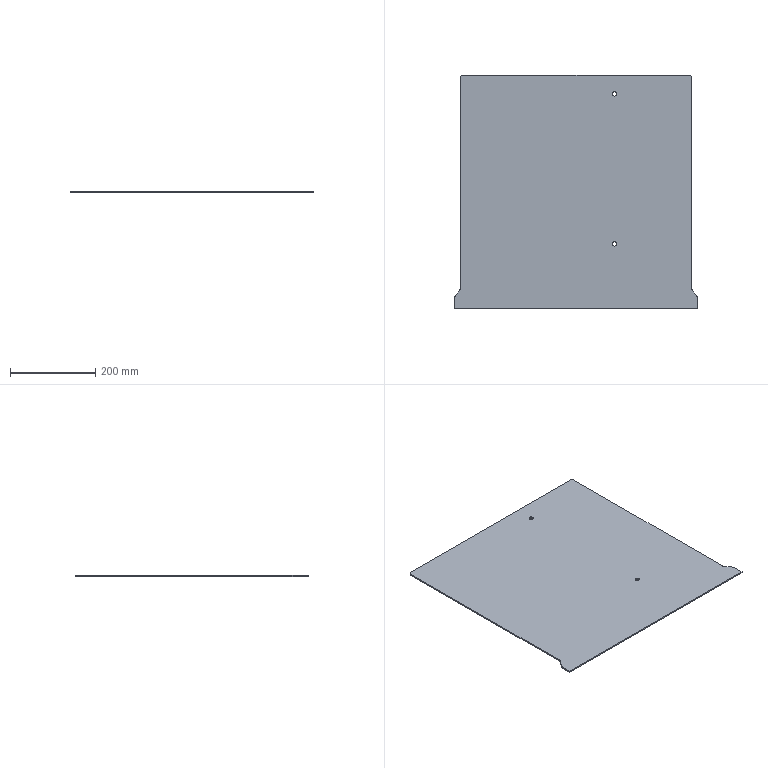Part | SolidWorks | features Fillet 2, FlatPattern 1, SMBaseFlange 1, SheetMetal 1 | 1 solid | 20 faces | box 570 x 547 x 3 mm | volume 888967 mm3 | cylinder 10 | plane 10 | commonest cylinder face diameters 10 x6 20 x4
STEP:
#1=CARTESIAN_POINT('',(370.,152.,-3.));
#2=VERTEX_POINT('',#1);
#3=CARTESIAN_POINT('',(380.,152.,-3.));
#4=VERTEX_POINT('',#3);
#5=CARTESIAN_POINT('',(375.,152.,-3.));
#6=DIRECTION('',(0.,0.,1.));
#7=DIRECTION('',(1.,0.,0.));
#8=AXIS2_PLACEMENT_3D('',#5,#6,#7);
#9=CIRCLE('',#8,5.);
#10=EDGE_CURVE('',#2,#4,#9,.T.);
#11=ORIENTED_EDGE('',*,*,#10,.F.);
#12=CARTESIAN_POINT('',(370.,152.,0.));
#13=VERTEX_POINT('',#12);
#14=CARTESIAN_POINT('',(370.,152.,-3.));
#15=DIRECTION('',(0.,0.,1.));
#16=VECTOR('',#15,1000.);
#17=LINE('',#14,#16);
#18=EDGE_CURVE('',#2,#13,#17,.T.);
#19=ORIENTED_EDGE('',*,*,#18,.T.);
#20=CARTESIAN_POINT('',(380.,152.,0.));
#21=VERTEX_POINT('',#20);
#22=CARTESIAN_POINT('',(375.,152.,0.));
#23=DIRECTION('',(0.,0.,1.));
#24=DIRECTION('',(1.,0.,0.));
#25=AXIS2_PLACEMENT_3D('',#22,#23,#24);
#26=CIRCLE('',#25,5.);
#27=EDGE_CURVE('',#13,#21,#26,.T.);
#28=ORIENTED_EDGE('',*,*,#27,.T.);
#29=CARTESIAN_POINT('',(380.,152.,-3.));
#30=DIRECTION('',(0.,0.,1.));
#31=VECTOR('',#30,1000.);
#32=LINE('',#29,#31);
#33=EDGE_CURVE('',#4,#21,#32,.T.);
#34=ORIENTED_EDGE('',*,*,#33,.F.);
#35=EDGE_LOOP('',(#11,#19,#28,#34));
#36=FACE_OUTER_BOUND('',#35,.T.);
#37=CARTESIAN_POINT('',(375.,152.,-3.));
#38=DIRECTION('',(0.,0.,1.));
#39=DIRECTION('',(1.,0.,0.));
#40=AXIS2_PLACEMENT_3D('',#37,#38,#39);
#41=CYLINDRICAL_SURFACE('',#40,5.);
#42=ADVANCED_FACE('',(#36),#41,.F.);
#43=CARTESIAN_POINT('',(370.,503.,-3.));
#44=VERTEX_POINT('',#43);
#45=CARTESIAN_POINT('',(380.,503.,-3.));
#46=VERTEX_POINT('',#45);
#47=CARTESIAN_POINT('',(375.,503.,-3.));
#48=DIRECTION('',(0.,0.,1.));
#49=DIRECTION('',(1.,0.,0.));
#50=AXIS2_PLACEMENT_3D('',#47,#48,#49);
#51=CIRCLE('',#50,5.);
#52=EDGE_CURVE('',#44,#46,#51,.T.);
#53=ORIENTED_EDGE('',*,*,#52,.F.);
#54=CARTESIAN_POINT('',(370.,503.,0.));
#55=VERTEX_POINT('',#54);
#56=CARTESIAN_POINT('',(370.,503.,-3.));
#57=DIRECTION('',(0.,0.,1.));
#58=VECTOR('',#57,1000.);
#59=LINE('',#56,#58);
#60=EDGE_CURVE('',#44,#55,#59,.T.);
#61=ORIENTED_EDGE('',*,*,#60,.T.);
#62=CARTESIAN_POINT('',(380.,503.,0.));
#63=VERTEX_POINT('',#62);
#64=CARTESIAN_POINT('',(375.,503.,0.));
#65=DIRECTION('',(0.,0.,1.));
#66=DIRECTION('',(1.,0.,0.));
#67=AXIS2_PLACEMENT_3D('',#64,#65,#66);
#68=CIRCLE('',#67,5.);
#69=EDGE_CURVE('',#55,#63,#68,.T.);
#70=ORIENTED_EDGE('',*,*,#69,.T.);
#71=CARTESIAN_POINT('',(380.,503.,-3.));
#72=DIRECTION('',(0.,0.,1.));
#73=VECTOR('',#72,1000.);
#74=LINE('',#71,#73);
#75=EDGE_CURVE('',#46,#63,#74,.T.);
#76=ORIENTED_EDGE('',*,*,#75,.F.);
#77=EDGE_LOOP('',(#53,#61,#70,#76));
#78=FACE_OUTER_BOUND('',#77,.T.);
#79=CARTESIAN_POINT('',(375.,503.,-3.));
#80=DIRECTION('',(0.,0.,1.));
#81=DIRECTION('',(1.,0.,0.));
#82=AXIS2_PLACEMENT_3D('',#79,#80,#81);
#83=CYLINDRICAL_SURFACE('',#82,5.);
#84=ADVANCED_FACE('',(#78),#83,.F.);
#85=CARTESIAN_POINT('',(0.,23.667,0.));
#86=VERTEX_POINT('',#85);
#87=CARTESIAN_POINT('',(0.,0.,0.));
#88=VERTEX_POINT('',#87);
#89=CARTESIAN_POINT('',(0.,0.,0.));
#90=DIRECTION('',(0.,-1.,0.));
#91=VECTOR('',#90,1000.);
#92=LINE('',#89,#91);
#93=EDGE_CURVE('',#86,#88,#92,.T.);
#94=ORIENTED_EDGE('',*,*,#93,.F.);
#95=CARTESIAN_POINT('',(0.,23.667,-3.));
#96=VERTEX_POINT('',#95);
#97=CARTESIAN_POINT('',(0.,23.667,-3.));
#98=DIRECTION('',(0.,0.,-1.));
#99=VECTOR('',#98,1000.);
#100=LINE('',#97,#99);
#101=EDGE_CURVE('',#86,#96,#100,.T.);
#102=ORIENTED_EDGE('',*,*,#101,.T.);
#103=CARTESIAN_POINT('',(0.,0.,-3.));
#104=VERTEX_POINT('',#103);
#105=CARTESIAN_POINT('',(0.,0.,-3.));
#106=DIRECTION('',(0.,-1.,0.));
#107=VECTOR('',#106,1000.);
#108=LINE('',#105,#107);
#109=EDGE_CURVE('',#96,#104,#108,.T.);
#110=ORIENTED_EDGE('',*,*,#109,.T.);
#111=CARTESIAN_POINT('',(0.,0.,-3.));
#112=DIRECTION('',(0.,0.,1.));
#113=VECTOR('',#112,1000.);
#114=LINE('',#111,#113);
#115=EDGE_CURVE('',#104,#88,#114,.T.);
#116=ORIENTED_EDGE('',*,*,#115,.T.);
#117=EDGE_LOOP('',(#94,#102,#110,#116));
#118=FACE_OUTER_BOUND('',#117,.T.);
#119=CARTESIAN_POINT('',(0.,0.,-3.));
#120=DIRECTION('',(-1.,0.,0.));
#121=DIRECTION('',(0.,0.,1.));
#122=AXIS2_PLACEMENT_3D('',#119,#120,#121);
#123=PLANE('',#122);
#124=ADVANCED_FACE('',(#118),#123,.T.);
#125=CARTESIAN_POINT('',(13.,44.333,-3.));
#126=VERTEX_POINT('',#125);
#127=CARTESIAN_POINT('',(2.,29.667,-3.));
#128=VERTEX_POINT('',#127);
#129=CARTESIAN_POINT('',(15.,47.,-3.));
#130=DIRECTION('',(-0.6,-0.8,0.));
#131=VECTOR('',#130,1000.);
#132=LINE('',#129,#131);
#133=EDGE_CURVE('',#126,#128,#132,.T.);
#134=ORIENTED_EDGE('',*,*,#133,.T.);
#135=CARTESIAN_POINT('',(2.,29.667,0.));
#136=VERTEX_POINT('',#135);
#137=CARTESIAN_POINT('',(2.,29.667,-3.));
#138=DIRECTION('',(0.,0.,1.));
#139=VECTOR('',#138,1000.);
#140=LINE('',#137,#139);
#141=EDGE_CURVE('',#128,#136,#140,.T.);
#142=ORIENTED_EDGE('',*,*,#141,.T.);
#143=CARTESIAN_POINT('',(13.,44.333,0.));
#144=VERTEX_POINT('',#143);
#145=CARTESIAN_POINT('',(15.,47.,0.));
#146=DIRECTION('',(-0.6,-0.8,0.));
#147=VECTOR('',#146,1000.);
#148=LINE('',#145,#147);
#149=EDGE_CURVE('',#144,#136,#148,.T.);
#150=ORIENTED_EDGE('',*,*,#149,.F.);
#151=CARTESIAN_POINT('',(13.,44.333,-3.));
#152=DIRECTION('',(0.,0.,-1.));
#153=VECTOR('',#152,1000.);
#154=LINE('',#151,#153);
#155=EDGE_CURVE('',#144,#126,#154,.T.);
#156=ORIENTED_EDGE('',*,*,#155,.T.);
#157=EDGE_LOOP('',(#134,#142,#150,#156));
#158=FACE_OUTER_BOUND('',#157,.T.);
#159=CARTESIAN_POINT('',(15.,47.,-3.));
#160=DIRECTION('',(-0.8,0.6,0.));
#161=DIRECTION('',(-0.6,-0.8,0.));
#162=AXIS2_PLACEMENT_3D('',#159,#160,#161);
#163=PLANE('',#162);
#164=ADVANCED_FACE('',(#158),#163,.T.);
#165=CARTESIAN_POINT('',(15.,542.,0.));
#166=VERTEX_POINT('',#165);
#167=CARTESIAN_POINT('',(15.,50.333,0.));
#168=VERTEX_POINT('',#167);
#169=CARTESIAN_POINT('',(15.,547.,0.));
#170=DIRECTION('',(0.,-1.,0.));
#171=VECTOR('',#170,1000.);
#172=LINE('',#169,#171);
#173=EDGE_CURVE('',#166,#168,#172,.T.);
#174=ORIENTED_EDGE('',*,*,#173,.F.);
#175=CARTESIAN_POINT('',(15.,542.,-3.));
#176=VERTEX_POINT('',#175);
#177=CARTESIAN_POINT('',(15.,542.,-3.));
#178=DIRECTION('',(0.,0.,-1.));
#179=VECTOR('',#178,1000.);
#180=LINE('',#177,#179);
#181=EDGE_CURVE('',#166,#176,#180,.T.);
#182=ORIENTED_EDGE('',*,*,#181,.T.);
#183=CARTESIAN_POINT('',(15.,50.333,-3.));
#184=VERTEX_POINT('',#183);
#185=CARTESIAN_POINT('',(15.,547.,-3.));
#186=DIRECTION('',(0.,-1.,0.));
#187=VECTOR('',#186,1000.);
#188=LINE('',#185,#187);
#189=EDGE_CURVE('',#176,#184,#188,.T.);
#190=ORIENTED_EDGE('',*,*,#189,.T.);
#191=CARTESIAN_POINT('',(15.,50.333,0.));
#192=DIRECTION('',(0.,0.,1.));
#193=VECTOR('',#192,1000.);
#194=LINE('',#191,#193);
#195=EDGE_CURVE('',#184,#168,#194,.T.);
#196=ORIENTED_EDGE('',*,*,#195,.T.);
#197=EDGE_LOOP('',(#174,#182,#190,#196));
#198=FACE_OUTER_BOUND('',#197,.T.);
#199=CARTESIAN_POINT('',(15.,547.,-3.));
#200=DIRECTION('',(-1.,0.,0.));
#201=DIRECTION('',(0.,-1.,0.));
#202=AXIS2_PLACEMENT_3D('',#199,#200,#201);
#203=PLANE('',#202);
#204=ADVANCED_FACE('',(#198),#203,.T.);
#205=CARTESIAN_POINT('',(550.,547.,0.));
#206=VERTEX_POINT('',#205);
#207=CARTESIAN_POINT('',(20.,547.,0.));
#208=VERTEX_POINT('',#207);
#209=CARTESIAN_POINT('',(15.,547.,0.));
#210=DIRECTION('',(-1.,0.,0.));
#211=VECTOR('',#210,1000.);
#212=LINE('',#209,#211);
#213=EDGE_CURVE('',#206,#208,#212,.T.);
#214=ORIENTED_EDGE('',*,*,#213,.F.);
#215=CARTESIAN_POINT('',(550.,547.,-3.));
#216=VERTEX_POINT('',#215);
#217=CARTESIAN_POINT('',(550.,547.,-3.));
#218=DIRECTION('',(0.,0.,-1.));
#219=VECTOR('',#218,1000.);
#220=LINE('',#217,#219);
#221=EDGE_CURVE('',#206,#216,#220,.T.);
#222=ORIENTED_EDGE('',*,*,#221,.T.);
#223=CARTESIAN_POINT('',(20.,547.,-3.));
#224=VERTEX_POINT('',#223);
#225=CARTESIAN_POINT('',(15.,547.,-3.));
#226=DIRECTION('',(-1.,0.,0.));
#227=VECTOR('',#226,1000.);
#228=LINE('',#225,#227);
#229=EDGE_CURVE('',#216,#224,#228,.T.);
#230=ORIENTED_EDGE('',*,*,#229,.T.);
#231=CARTESIAN_POINT('',(20.,547.,-3.));
#232=DIRECTION('',(0.,0.,1.));
#233=VECTOR('',#232,1000.);
#234=LINE('',#231,#233);
#235=EDGE_CURVE('',#224,#208,#234,.T.);
#236=ORIENTED_EDGE('',*,*,#235,.T.);
#237=EDGE_LOOP('',(#214,#222,#230,#236));
#238=FACE_OUTER_BOUND('',#237,.T.);
#239=CARTESIAN_POINT('',(15.,547.,-3.));
#240=DIRECTION('',(0.,1.,0.));
#241=DIRECTION('',(-1.,0.,0.));
#242=AXIS2_PLACEMENT_3D('',#239,#240,#241);
#243=PLANE('',#242);
#244=ADVANCED_FACE('',(#238),#243,.T.);
#245=CARTESIAN_POINT('',(555.,50.333,-3.));
#246=VERTEX_POINT('',#245);
#247=CARTESIAN_POINT('',(555.,542.,-3.));
#248=VERTEX_POINT('',#247);
#249=CARTESIAN_POINT('',(555.,547.,-3.));
#250=DIRECTION('',(0.,1.,0.));
#251=VECTOR('',#250,1000.);
#252=LINE('',#249,#251);
#253=EDGE_CURVE('',#246,#248,#252,.T.);
#254=ORIENTED_EDGE('',*,*,#253,.T.);
#255=CARTESIAN_POINT('',(555.,542.,0.));
#256=VERTEX_POINT('',#255);
#257=CARTESIAN_POINT('',(555.,542.,-3.));
#258=DIRECTION('',(0.,0.,1.));
#259=VECTOR('',#258,1000.);
#260=LINE('',#257,#259);
#261=EDGE_CURVE('',#248,#256,#260,.T.);
#262=ORIENTED_EDGE('',*,*,#261,.T.);
#263=CARTESIAN_POINT('',(555.,50.333,0.));
#264=VERTEX_POINT('',#263);
#265=CARTESIAN_POINT('',(555.,547.,0.));
#266=DIRECTION('',(0.,1.,0.));
#267=VECTOR('',#266,1000.);
#268=LINE('',#265,#267);
#269=EDGE_CURVE('',#264,#256,#268,.T.);
#270=ORIENTED_EDGE('',*,*,#269,.F.);
#271=CARTESIAN_POINT('',(555.,50.333,-3.));
#272=DIRECTION('',(0.,0.,-1.));
#273=VECTOR('',#272,1000.);
#274=LINE('',#271,#273);
#275=EDGE_CURVE('',#264,#246,#274,.T.);
#276=ORIENTED_EDGE('',*,*,#275,.T.);
#277=EDGE_LOOP('',(#254,#262,#270,#276));
#278=FACE_OUTER_BOUND('',#277,.T.);
#279=CARTESIAN_POINT('',(555.,547.,-3.));
#280=DIRECTION('',(1.,0.,0.));
#281=DIRECTION('',(0.,1.,0.));
#282=AXIS2_PLACEMENT_3D('',#279,#280,#281);
#283=PLANE('',#282);
#284=ADVANCED_FACE('',(#278),#283,.T.);
#285=CARTESIAN_POINT('',(568.,29.667,0.));
#286=VERTEX_POINT('',#285);
#287=CARTESIAN_POINT('',(557.,44.333,0.));
#288=VERTEX_POINT('',#287);
#289=CARTESIAN_POINT('',(555.,47.,0.));
#290=DIRECTION('',(-0.6,0.8,0.));
#291=VECTOR('',#290,1000.);
#292=LINE('',#289,#291);
#293=EDGE_CURVE('',#286,#288,#292,.T.);
#294=ORIENTED_EDGE('',*,*,#293,.F.);
#295=CARTESIAN_POINT('',(568.,29.667,-3.));
#296=VERTEX_POINT('',#295);
#297=CARTESIAN_POINT('',(568.,29.667,-3.));
#298=DIRECTION('',(0.,0.,-1.));
#299=VECTOR('',#298,1000.);
#300=LINE('',#297,#299);
#301=EDGE_CURVE('',#286,#296,#300,.T.);
#302=ORIENTED_EDGE('',*,*,#301,.T.);
#303=CARTESIAN_POINT('',(557.,44.333,-3.));
#304=VERTEX_POINT('',#303);
#305=CARTESIAN_POINT('',(555.,47.,-3.));
#306=DIRECTION('',(-0.6,0.8,0.));
#307=VECTOR('',#306,1000.);
#308=LINE('',#305,#307);
#309=EDGE_CURVE('',#296,#304,#308,.T.);
#310=ORIENTED_EDGE('',*,*,#309,.T.);
#311=CARTESIAN_POINT('',(557.,44.333,0.));
#312=DIRECTION('',(0.,0.,1.));
#313=VECTOR('',#312,1000.);
#314=LINE('',#311,#313);
#315=EDGE_CURVE('',#304,#288,#314,.T.);
#316=ORIENTED_EDGE('',*,*,#315,.T.);
#317=EDGE_LOOP('',(#294,#302,#310,#316));
#318=FACE_OUTER_BOUND('',#317,.T.);
#319=CARTESIAN_POINT('',(555.,47.,-3.));
#320=DIRECTION('',(0.8,0.6,0.));
#321=DIRECTION('',(-0.6,0.8,0.));
#322=AXIS2_PLACEMENT_3D('',#319,#320,#321);
#323=PLANE('',#322);
#324=ADVANCED_FACE('',(#318),#323,.T.);
#325=CARTESIAN_POINT('',(570.,0.,-3.));
#326=VERTEX_POINT('',#325);
#327=CARTESIAN_POINT('',(570.,23.667,-3.));
#328=VERTEX_POINT('',#327);
#329=CARTESIAN_POINT('',(570.,0.,-3.));
#330=DIRECTION('',(0.,1.,0.));
#331=VECTOR('',#330,1000.);
#332=LINE('',#329,#331);
#333=EDGE_CURVE('',#326,#328,#332,.T.);
#334=ORIENTED_EDGE('',*,*,#333,.T.);
#335=CARTESIAN_POINT('',(570.,23.667,0.));
#336=VERTEX_POINT('',#335);
#337=CARTESIAN_POINT('',(570.,23.667,-3.));
#338=DIRECTION('',(0.,0.,1.));
#339=VECTOR('',#338,1000.);
#340=LINE('',#337,#339);
#341=EDGE_CURVE('',#328,#336,#340,.T.);
#342=ORIENTED_EDGE('',*,*,#341,.T.);
#343=CARTESIAN_POINT('',(570.,0.,0.));
#344=VERTEX_POINT('',#343);
#345=CARTESIAN_POINT('',(570.,0.,0.));
#346=DIRECTION('',(0.,1.,0.));
#347=VECTOR('',#346,1000.);
#348=LINE('',#345,#347);
#349=EDGE_CURVE('',#344,#336,#348,.T.);
#350=ORIENTED_EDGE('',*,*,#349,.F.);
#351=CARTESIAN_POINT('',(570.,0.,-3.));
#352=DIRECTION('',(0.,0.,1.));
#353=VECTOR('',#352,1000.);
#354=LINE('',#351,#353);
#355=EDGE_CURVE('',#326,#344,#354,.T.);
#356=ORIENTED_EDGE('',*,*,#355,.F.);
#357=EDGE_LOOP('',(#334,#342,#350,#356));
#358=FACE_OUTER_BOUND('',#357,.T.);
#359=CARTESIAN_POINT('',(570.,0.,-3.));
#360=DIRECTION('',(1.,0.,0.));
#361=DIRECTION('',(0.,0.,-1.));
#362=AXIS2_PLACEMENT_3D('',#359,#360,#361);
#363=PLANE('',#362);
#364=ADVANCED_FACE('',(#358),#363,.T.);
#365=CARTESIAN_POINT('',(0.,0.,0.));
#366=DIRECTION('',(1.,0.,0.));
#367=VECTOR('',#366,1000.);
#368=LINE('',#365,#367);
#369=EDGE_CURVE('',#88,#344,#368,.T.);
#370=ORIENTED_EDGE('',*,*,#369,.F.);
#371=ORIENTED_EDGE('',*,*,#115,.F.);
#372=CARTESIAN_POINT('',(0.,0.,-3.));
#373=DIRECTION('',(1.,0.,0.));
#374=VECTOR('',#373,1000.);
#375=LINE('',#372,#374);
#376=EDGE_CURVE('',#104,#326,#375,.T.);
#377=ORIENTED_EDGE('',*,*,#376,.T.);
#378=ORIENTED_EDGE('',*,*,#355,.T.);
#379=EDGE_LOOP('',(#370,#371,#377,#378));
#380=FACE_OUTER_BOUND('',#379,.T.);
#381=CARTESIAN_POINT('',(0.,0.,-3.));
#382=DIRECTION('',(0.,-1.,0.));
#383=DIRECTION('',(0.,0.,-1.));
#384=AXIS2_PLACEMENT_3D('',#381,#382,#383);
#385=PLANE('',#384);
#386=ADVANCED_FACE('',(#380),#385,.T.);
#387=CARTESIAN_POINT('',(375.,152.,-3.));
#388=DIRECTION('',(0.,0.,1.));
#389=DIRECTION('',(1.,0.,0.));
#390=AXIS2_PLACEMENT_3D('',#387,#388,#389);
#391=CIRCLE('',#390,5.);
#392=EDGE_CURVE('',#4,#2,#391,.T.);
#393=ORIENTED_EDGE('',*,*,#392,.T.);
#394=ORIENTED_EDGE('',*,*,#10,.T.);
#395=EDGE_LOOP('',(#393,#394));
#396=FACE_BOUND('',#395,.T.);
#397=CARTESIAN_POINT('',(375.,503.,-3.));
#398=DIRECTION('',(0.,0.,1.));
#399=DIRECTION('',(1.,0.,0.));
#400=AXIS2_PLACEMENT_3D('',#397,#398,#399);
#401=CIRCLE('',#400,5.);
#402=EDGE_CURVE('',#46,#44,#401,.T.);
#403=ORIENTED_EDGE('',*,*,#402,.T.);
#404=ORIENTED_EDGE('',*,*,#52,.T.);
#405=EDGE_LOOP('',(#403,#404));
#406=FACE_BOUND('',#405,.T.);
#407=ORIENTED_EDGE('',*,*,#229,.F.);
#408=CARTESIAN_POINT('',(550.,542.,-3.));
#409=DIRECTION('',(0.,0.,-1.));
#410=DIRECTION('',(-1.,0.,0.));
#411=AXIS2_PLACEMENT_3D('',#408,#409,#410);
#412=CIRCLE('',#411,5.);
#413=EDGE_CURVE('',#216,#248,#412,.T.);
#414=ORIENTED_EDGE('',*,*,#413,.T.);
#415=ORIENTED_EDGE('',*,*,#253,.F.);
#416=CARTESIAN_POINT('',(565.,50.333,-3.));
#417=DIRECTION('',(0.,0.,1.));
#418=DIRECTION('',(-1.,0.,0.));
#419=AXIS2_PLACEMENT_3D('',#416,#417,#418);
#420=CIRCLE('',#419,10.);
#421=EDGE_CURVE('',#246,#304,#420,.T.);
#422=ORIENTED_EDGE('',*,*,#421,.T.);
#423=ORIENTED_EDGE('',*,*,#309,.F.);
#424=CARTESIAN_POINT('',(560.,23.667,-3.));
#425=DIRECTION('',(0.,0.,-1.));
#426=DIRECTION('',(-1.,0.,0.));
#427=AXIS2_PLACEMENT_3D('',#424,#425,#426);
#428=CIRCLE('',#427,10.);
#429=EDGE_CURVE('',#296,#328,#428,.T.);
#430=ORIENTED_EDGE('',*,*,#429,.T.);
#431=ORIENTED_EDGE('',*,*,#333,.F.);
#432=ORIENTED_EDGE('',*,*,#376,.F.);
#433=ORIENTED_EDGE('',*,*,#109,.F.);
#434=CARTESIAN_POINT('',(10.,23.667,-3.));
#435=DIRECTION('',(0.,0.,-1.));
#436=DIRECTION('',(-1.,0.,0.));
#437=AXIS2_PLACEMENT_3D('',#434,#435,#436);
#438=CIRCLE('',#437,10.);
#439=EDGE_CURVE('',#96,#128,#438,.T.);
#440=ORIENTED_EDGE('',*,*,#439,.T.);
#441=ORIENTED_EDGE('',*,*,#133,.F.);
#442=CARTESIAN_POINT('',(5.,50.333,-3.));
#443=DIRECTION('',(0.,0.,1.));
#444=DIRECTION('',(-1.,0.,0.));
#445=AXIS2_PLACEMENT_3D('',#442,#443,#444);
#446=CIRCLE('',#445,10.);
#447=EDGE_CURVE('',#126,#184,#446,.T.);
#448=ORIENTED_EDGE('',*,*,#447,.T.);
#449=ORIENTED_EDGE('',*,*,#189,.F.);
#450=CARTESIAN_POINT('',(20.,542.,-3.));
#451=DIRECTION('',(0.,0.,-1.));
#452=DIRECTION('',(-1.,0.,0.));
#453=AXIS2_PLACEMENT_3D('',#450,#451,#452);
#454=CIRCLE('',#453,5.);
#455=EDGE_CURVE('',#176,#224,#454,.T.);
#456=ORIENTED_EDGE('',*,*,#455,.T.);
#457=EDGE_LOOP('',(#407,#414,#415,#422,#423,#430,#431,#432,#433,#440,#441,#448,#449,#456));
#458=FACE_OUTER_BOUND('',#457,.T.);
#459=CARTESIAN_POINT('',(0.,0.,-3.));
#460=DIRECTION('',(0.,0.,-1.));
#461=DIRECTION('',(-1.,0.,0.));
#462=AXIS2_PLACEMENT_3D('',#459,#460,#461);
#463=PLANE('',#462);
#464=ADVANCED_FACE('',(#396,#406,#458),#463,.T.);
#465=CARTESIAN_POINT('',(375.,152.,0.));
#466=DIRECTION('',(0.,0.,1.));
#467=DIRECTION('',(1.,0.,0.));
#468=AXIS2_PLACEMENT_3D('',#465,#466,#467);
#469=CIRCLE('',#468,5.);
#470=EDGE_CURVE('',#21,#13,#469,.T.);
#471=ORIENTED_EDGE('',*,*,#470,.F.);
#472=ORIENTED_EDGE('',*,*,#27,.F.);
#473=EDGE_LOOP('',(#471,#472));
#474=FACE_BOUND('',#473,.T.);
#475=CARTESIAN_POINT('',(375.,503.,0.));
#476=DIRECTION('',(0.,0.,1.));
#477=DIRECTION('',(1.,0.,0.));
#478=AXIS2_PLACEMENT_3D('',#475,#476,#477);
#479=CIRCLE('',#478,5.);
#480=EDGE_CURVE('',#63,#55,#479,.T.);
#481=ORIENTED_EDGE('',*,*,#480,.F.);
#482=ORIENTED_EDGE('',*,*,#69,.F.);
#483=EDGE_LOOP('',(#481,#482));
#484=FACE_BOUND('',#483,.T.);
#485=ORIENTED_EDGE('',*,*,#269,.T.);
#486=CARTESIAN_POINT('',(550.,542.,0.));
#487=DIRECTION('',(0.,0.,1.));
#488=DIRECTION('',(-1.,0.,0.));
#489=AXIS2_PLACEMENT_3D('',#486,#487,#488);
#490=CIRCLE('',#489,5.);
#491=EDGE_CURVE('',#256,#206,#490,.T.);
#492=ORIENTED_EDGE('',*,*,#491,.T.);
#493=ORIENTED_EDGE('',*,*,#213,.T.);
#494=CARTESIAN_POINT('',(20.,542.,0.));
#495=DIRECTION('',(0.,0.,1.));
#496=DIRECTION('',(-1.,0.,0.));
#497=AXIS2_PLACEMENT_3D('',#494,#495,#496);
#498=CIRCLE('',#497,5.);
#499=EDGE_CURVE('',#208,#166,#498,.T.);
#500=ORIENTED_EDGE('',*,*,#499,.T.);
#501=ORIENTED_EDGE('',*,*,#173,.T.);
#502=CARTESIAN_POINT('',(5.,50.333,0.));
#503=DIRECTION('',(0.,0.,-1.));
#504=DIRECTION('',(-1.,0.,0.));
#505=AXIS2_PLACEMENT_3D('',#502,#503,#504);
#506=CIRCLE('',#505,10.);
#507=EDGE_CURVE('',#168,#144,#506,.T.);
#508=ORIENTED_EDGE('',*,*,#507,.T.);
#509=ORIENTED_EDGE('',*,*,#149,.T.);
#510=CARTESIAN_POINT('',(10.,23.667,0.));
#511=DIRECTION('',(0.,0.,1.));
#512=DIRECTION('',(-1.,0.,0.));
#513=AXIS2_PLACEMENT_3D('',#510,#511,#512);
#514=CIRCLE('',#513,10.);
#515=EDGE_CURVE('',#136,#86,#514,.T.);
#516=ORIENTED_EDGE('',*,*,#515,.T.);
#517=ORIENTED_EDGE('',*,*,#93,.T.);
#518=ORIENTED_EDGE('',*,*,#369,.T.);
#519=ORIENTED_EDGE('',*,*,#349,.T.);
#520=CARTESIAN_POINT('',(560.,23.667,0.));
#521=DIRECTION('',(0.,0.,1.));
#522=DIRECTION('',(-1.,0.,0.));
#523=AXIS2_PLACEMENT_3D('',#520,#521,#522);
#524=CIRCLE('',#523,10.);
#525=EDGE_CURVE('',#336,#286,#524,.T.);
#526=ORIENTED_EDGE('',*,*,#525,.T.);
#527=ORIENTED_EDGE('',*,*,#293,.T.);
#528=CARTESIAN_POINT('',(565.,50.333,0.));
#529=DIRECTION('',(0.,0.,-1.));
#530=DIRECTION('',(-1.,0.,0.));
#531=AXIS2_PLACEMENT_3D('',#528,#529,#530);
#532=CIRCLE('',#531,10.);
#533=EDGE_CURVE('',#288,#264,#532,.T.);
#534=ORIENTED_EDGE('',*,*,#533,.T.);
#535=EDGE_LOOP('',(#485,#492,#493,#500,#501,#508,#509,#516,#517,#518,#519,#526,#527,#534));
#536=FACE_OUTER_BOUND('',#535,.T.);
#537=CARTESIAN_POINT('',(0.,0.,0.));
#538=DIRECTION('',(0.,0.,-1.));
#539=DIRECTION('',(-1.,0.,0.));
#540=AXIS2_PLACEMENT_3D('',#537,#538,#539);
#541=PLANE('',#540);
#542=ADVANCED_FACE('',(#474,#484,#536),#541,.F.);
#543=ORIENTED_EDGE('',*,*,#60,.F.);
#544=ORIENTED_EDGE('',*,*,#402,.F.);
#545=ORIENTED_EDGE('',*,*,#75,.T.);
#546=ORIENTED_EDGE('',*,*,#480,.T.);
#547=EDGE_LOOP('',(#543,#544,#545,#546));
#548=FACE_OUTER_BOUND('',#547,.T.);
#549=CARTESIAN_POINT('',(375.,503.,-3.));
#550=DIRECTION('',(0.,0.,1.));
#551=DIRECTION('',(1.,0.,0.));
#552=AXIS2_PLACEMENT_3D('',#549,#550,#551);
#553=CYLINDRICAL_SURFACE('',#552,5.);
#554=ADVANCED_FACE('',(#548),#553,.F.);
#555=ORIENTED_EDGE('',*,*,#18,.F.);
#556=ORIENTED_EDGE('',*,*,#392,.F.);
#557=ORIENTED_EDGE('',*,*,#33,.T.);
#558=ORIENTED_EDGE('',*,*,#470,.T.);
#559=EDGE_LOOP('',(#555,#556,#557,#558));
#560=FACE_OUTER_BOUND('',#559,.T.);
#561=CARTESIAN_POINT('',(375.,152.,-3.));
#562=DIRECTION('',(0.,0.,1.));
#563=DIRECTION('',(1.,0.,0.));
#564=AXIS2_PLACEMENT_3D('',#561,#562,#563);
#565=CYLINDRICAL_SURFACE('',#564,5.);
#566=ADVANCED_FACE('',(#560),#565,.F.);
#567=ORIENTED_EDGE('',*,*,#429,.F.);
#568=ORIENTED_EDGE('',*,*,#301,.F.);
#569=ORIENTED_EDGE('',*,*,#525,.F.);
#570=ORIENTED_EDGE('',*,*,#341,.F.);
#571=EDGE_LOOP('',(#567,#568,#569,#570));
#572=FACE_OUTER_BOUND('',#571,.T.);
#573=CARTESIAN_POINT('',(560.,23.667,-3.));
#574=DIRECTION('',(0.,0.,1.));
#575=DIRECTION('',(1.,0.,0.));
#576=AXIS2_PLACEMENT_3D('',#573,#574,#575);
#577=CYLINDRICAL_SURFACE('',#576,10.);
#578=ADVANCED_FACE('',(#572),#577,.T.);
#579=ORIENTED_EDGE('',*,*,#421,.F.);
#580=ORIENTED_EDGE('',*,*,#275,.F.);
#581=ORIENTED_EDGE('',*,*,#533,.F.);
#582=ORIENTED_EDGE('',*,*,#315,.F.);
#583=EDGE_LOOP('',(#579,#580,#581,#582));
#584=FACE_OUTER_BOUND('',#583,.T.);
#585=CARTESIAN_POINT('',(565.,50.333,-3.));
#586=DIRECTION('',(0.,0.,-1.));
#587=DIRECTION('',(-1.,0.,0.));
#588=AXIS2_PLACEMENT_3D('',#585,#586,#587);
#589=CYLINDRICAL_SURFACE('',#588,10.);
#590=ADVANCED_FACE('',(#584),#589,.F.);
#591=ORIENTED_EDGE('',*,*,#439,.F.);
#592=ORIENTED_EDGE('',*,*,#101,.F.);
#593=ORIENTED_EDGE('',*,*,#515,.F.);
#594=ORIENTED_EDGE('',*,*,#141,.F.);
#595=EDGE_LOOP('',(#591,#592,#593,#594));
#596=FACE_OUTER_BOUND('',#595,.T.);
#597=CARTESIAN_POINT('',(10.,23.667,-3.));
#598=DIRECTION('',(0.,0.,1.));
#599=DIRECTION('',(1.,0.,0.));
#600=AXIS2_PLACEMENT_3D('',#597,#598,#599);
#601=CYLINDRICAL_SURFACE('',#600,10.);
#602=ADVANCED_FACE('',(#596),#601,.T.);
#603=ORIENTED_EDGE('',*,*,#447,.F.);
#604=ORIENTED_EDGE('',*,*,#155,.F.);
#605=ORIENTED_EDGE('',*,*,#507,.F.);
#606=ORIENTED_EDGE('',*,*,#195,.F.);
#607=EDGE_LOOP('',(#603,#604,#605,#606));
#608=FACE_OUTER_BOUND('',#607,.T.);
#609=CARTESIAN_POINT('',(5.,50.333,-3.));
#610=DIRECTION('',(0.,0.,-1.));
#611=DIRECTION('',(-1.,0.,0.));
#612=AXIS2_PLACEMENT_3D('',#609,#610,#611);
#613=CYLINDRICAL_SURFACE('',#612,10.);
#614=ADVANCED_FACE('',(#608),#613,.F.);
#615=ORIENTED_EDGE('',*,*,#413,.F.);
#616=ORIENTED_EDGE('',*,*,#221,.F.);
#617=ORIENTED_EDGE('',*,*,#491,.F.);
#618=ORIENTED_EDGE('',*,*,#261,.F.);
#619=EDGE_LOOP('',(#615,#616,#617,#618));
#620=FACE_OUTER_BOUND('',#619,.T.);
#621=CARTESIAN_POINT('',(550.,542.,-3.));
#622=DIRECTION('',(0.,0.,1.));
#623=DIRECTION('',(1.,0.,0.));
#624=AXIS2_PLACEMENT_3D('',#621,#622,#623);
#625=CYLINDRICAL_SURFACE('',#624,5.);
#626=ADVANCED_FACE('',(#620),#625,.T.);
#627=ORIENTED_EDGE('',*,*,#455,.F.);
#628=ORIENTED_EDGE('',*,*,#181,.F.);
#629=ORIENTED_EDGE('',*,*,#499,.F.);
#630=ORIENTED_EDGE('',*,*,#235,.F.);
#631=EDGE_LOOP('',(#627,#628,#629,#630));
#632=FACE_OUTER_BOUND('',#631,.T.);
#633=CARTESIAN_POINT('',(20.,542.,-3.));
#634=DIRECTION('',(0.,0.,1.));
#635=DIRECTION('',(1.,0.,0.));
#636=AXIS2_PLACEMENT_3D('',#633,#634,#635);
#637=CYLINDRICAL_SURFACE('',#636,5.);
#638=ADVANCED_FACE('',(#632),#637,.T.);
#639=CLOSED_SHELL('',(#42,#84,#124,#164,#204,#244,#284,#324,#364,#386,#464,#542,#554,#566,#578,#590,#602,#614,#626,#638));
#640=MANIFOLD_SOLID_BREP('',#639);
#641=CARTESIAN_POINT('',(0.,0.,0.));
#642=DIRECTION('',(0.,0.,1.));
#643=DIRECTION('',(1.,0.,0.));
#644=AXIS2_PLACEMENT_3D('',#641,#642,#643);
#645=(LENGTH_UNIT()NAMED_UNIT(*)SI_UNIT(.MILLI.,.METRE.));
#646=UNCERTAINTY_MEASURE_WITH_UNIT(LENGTH_MEASURE(0.00001),#645,'','');
#647=(NAMED_UNIT(*)PLANE_ANGLE_UNIT()SI_UNIT($,.RADIAN.));
#648=(NAMED_UNIT(*)SI_UNIT($,.STERADIAN.)SOLID_ANGLE_UNIT());
#649=(GEOMETRIC_REPRESENTATION_CONTEXT(3)GLOBAL_UNCERTAINTY_ASSIGNED_CONTEXT((#646))GLOBAL_UNIT_ASSIGNED_CONTEXT((#645,#647,#648))REPRESENTATION_CONTEXT('',''));
#650=ADVANCED_BREP_SHAPE_REPRESENTATION('',(#640,#644),#649);